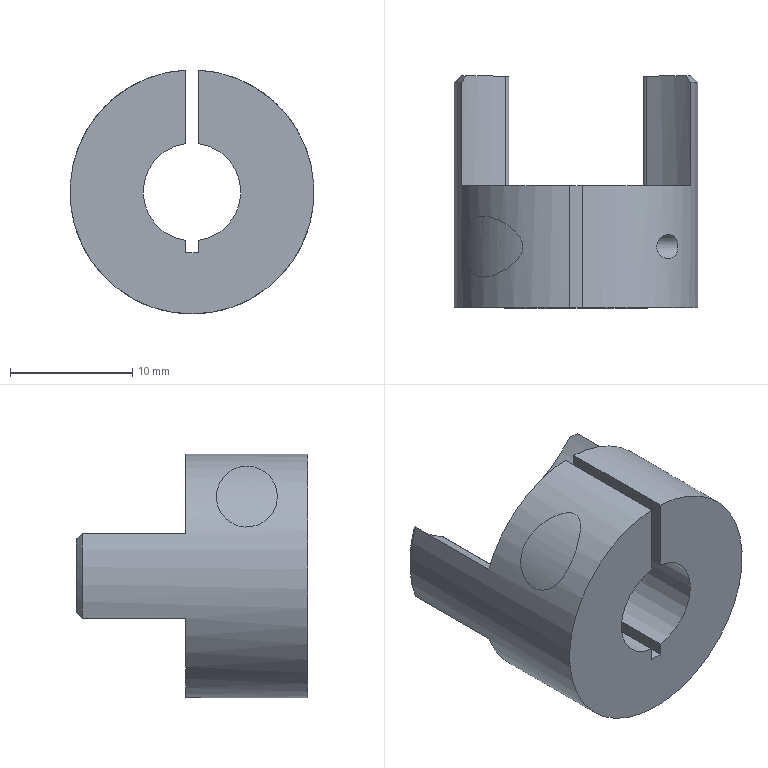Part | NX | features R-HUB_5003_022_GCJC20-BL-6-8 2 | 1 solid | 25 faces | box 20 x 19 x 19.987 mm | volume 2720 mm3 | cylinder 13 | plane 10 | cone 2 | commonest cylinder face diameters 24 x4 1 x2 8 x2 20 x2 2.013 x1 3 x1
STEP:
#1=CARTESIAN_POINT('',(-216.275,-588.6,-114.469));
#2=VERTEX_POINT('',#1);
#3=CARTESIAN_POINT('',(-216.275,-588.6,-106.531));
#4=VERTEX_POINT('',#3);
#5=CARTESIAN_POINT('',(-216.775,-588.6,-110.5));
#6=DIRECTION('',(0.,-1.,0.));
#7=DIRECTION('',(1.,0.,0.));
#8=AXIS2_PLACEMENT_3D('',#5,#6,#7);
#9=CIRCLE('',#8,4.);
#10=EDGE_CURVE('',#2,#4,#9,.T.);
#11=ORIENTED_EDGE('',*,*,#10,.T.);
#12=CARTESIAN_POINT('',(-216.275,-578.6,-106.531));
#13=VERTEX_POINT('',#12);
#14=CARTESIAN_POINT('',(-216.275,-569.599,-106.531));
#15=DIRECTION('',(0.,-1.,0.));
#16=VECTOR('',#15,1000.);
#17=LINE('',#14,#16);
#18=EDGE_CURVE('',#4,#13,#17,.F.);
#19=ORIENTED_EDGE('',*,*,#18,.T.);
#20=CARTESIAN_POINT('',(-216.275,-578.6,-114.469));
#21=VERTEX_POINT('',#20);
#22=CARTESIAN_POINT('',(-216.775,-578.6,-110.5));
#23=DIRECTION('',(0.,-1.,0.));
#24=DIRECTION('',(1.,0.,0.));
#25=AXIS2_PLACEMENT_3D('',#22,#23,#24);
#26=CIRCLE('',#25,4.);
#27=EDGE_CURVE('',#13,#21,#26,.F.);
#28=ORIENTED_EDGE('',*,*,#27,.T.);
#29=CARTESIAN_POINT('',(-216.275,-569.599,-114.469));
#30=DIRECTION('',(0.,-1.,0.));
#31=VECTOR('',#30,1000.);
#32=LINE('',#29,#31);
#33=EDGE_CURVE('',#21,#2,#32,.T.);
#34=ORIENTED_EDGE('',*,*,#33,.T.);
#35=EDGE_LOOP('',(#11,#19,#28,#34));
#36=FACE_BOUND('',#35,.T.);
#37=CARTESIAN_POINT('',(-216.775,-569.599,-110.5));
#38=DIRECTION('',(0.,-1.,0.));
#39=DIRECTION('',(1.,0.,0.));
#40=AXIS2_PLACEMENT_3D('',#37,#38,#39);
#41=CYLINDRICAL_SURFACE('',#40,4.);
#42=ADVANCED_FACE('',(#36),#41,.F.);
#43=CARTESIAN_POINT('',(-216.275,-588.6,-100.513));
#44=VERTEX_POINT('',#43);
#45=CARTESIAN_POINT('',(-217.275,-588.6,-100.513));
#46=VERTEX_POINT('',#45);
#47=CARTESIAN_POINT('',(-216.775,-588.6,-110.5));
#48=DIRECTION('',(0.,1.,0.));
#49=DIRECTION('',(-1.,0.,0.));
#50=AXIS2_PLACEMENT_3D('',#47,#48,#49);
#51=CIRCLE('',#50,10.);
#52=EDGE_CURVE('',#44,#46,#51,.T.);
#53=ORIENTED_EDGE('',*,*,#52,.F.);
#54=CARTESIAN_POINT('',(-216.275,-588.6,-110.5));
#55=DIRECTION('',(0.,0.,1.));
#56=VECTOR('',#55,1000.);
#57=LINE('',#54,#56);
#58=EDGE_CURVE('',#4,#44,#57,.T.);
#59=ORIENTED_EDGE('',*,*,#58,.F.);
#60=ORIENTED_EDGE('',*,*,#10,.F.);
#61=CARTESIAN_POINT('',(-216.275,-588.6,-115.5));
#62=VERTEX_POINT('',#61);
#63=CARTESIAN_POINT('',(-216.275,-588.6,-110.5));
#64=DIRECTION('',(0.,0.,1.));
#65=VECTOR('',#64,1000.);
#66=LINE('',#63,#65);
#67=EDGE_CURVE('',#62,#2,#66,.T.);
#68=ORIENTED_EDGE('',*,*,#67,.F.);
#69=CARTESIAN_POINT('',(-217.275,-588.6,-115.5));
#70=VERTEX_POINT('',#69);
#71=CARTESIAN_POINT('',(-216.775,-588.6,-115.5));
#72=DIRECTION('',(1.,0.,0.));
#73=VECTOR('',#72,1000.);
#74=LINE('',#71,#73);
#75=EDGE_CURVE('',#70,#62,#74,.T.);
#76=ORIENTED_EDGE('',*,*,#75,.F.);
#77=CARTESIAN_POINT('',(-217.275,-588.6,-114.469));
#78=VERTEX_POINT('',#77);
#79=CARTESIAN_POINT('',(-217.275,-588.6,-110.5));
#80=DIRECTION('',(0.,0.,-1.));
#81=VECTOR('',#80,1000.);
#82=LINE('',#79,#81);
#83=EDGE_CURVE('',#78,#70,#82,.T.);
#84=ORIENTED_EDGE('',*,*,#83,.F.);
#85=CARTESIAN_POINT('',(-217.275,-588.6,-106.531));
#86=VERTEX_POINT('',#85);
#87=CARTESIAN_POINT('',(-216.775,-588.6,-110.5));
#88=DIRECTION('',(0.,-1.,0.));
#89=DIRECTION('',(1.,0.,0.));
#90=AXIS2_PLACEMENT_3D('',#87,#88,#89);
#91=CIRCLE('',#90,4.);
#92=EDGE_CURVE('',#86,#78,#91,.T.);
#93=ORIENTED_EDGE('',*,*,#92,.F.);
#94=CARTESIAN_POINT('',(-217.275,-588.6,-110.5));
#95=DIRECTION('',(0.,0.,-1.));
#96=VECTOR('',#95,1000.);
#97=LINE('',#94,#96);
#98=EDGE_CURVE('',#46,#86,#97,.T.);
#99=ORIENTED_EDGE('',*,*,#98,.F.);
#100=EDGE_LOOP('',(#53,#59,#60,#68,#76,#84,#93,#99));
#101=FACE_BOUND('',#100,.T.);
#102=CARTESIAN_POINT('',(-216.775,-588.6,-110.5));
#103=DIRECTION('',(0.,1.,0.));
#104=DIRECTION('',(-1.,0.,0.));
#105=AXIS2_PLACEMENT_3D('',#102,#103,#104);
#106=PLANE('',#105);
#107=ADVANCED_FACE('',(#101),#106,.F.);
#108=CARTESIAN_POINT('',(-209.176,-584.606,-104.));
#109=VERTEX_POINT('',#108);
#110=CARTESIAN_POINT('',(-208.586,-584.456,-104.743));
#111=CARTESIAN_POINT('',(-209.17,-584.677,-103.982));
#112=CARTESIAN_POINT('',(-209.789,-584.474,-103.328));
#113=CARTESIAN_POINT('',(-210.332,-583.676,-102.85));
#114=CARTESIAN_POINT('',(-209.879,-582.783,-103.244));
#115=CARTESIAN_POINT('',(-209.245,-582.531,-103.895));
#116=CARTESIAN_POINT('',(-208.657,-582.678,-104.64));
#117=CARTESIAN_POINT('',(-208.32,-583.521,-105.161));
#118=CARTESIAN_POINT('',(-208.586,-584.456,-104.743));
#119=CARTESIAN_POINT('',(-209.17,-584.677,-103.982));
#120=CARTESIAN_POINT('',(-209.789,-584.474,-103.328));
#121=B_SPLINE_CURVE_WITH_KNOTS('',3,(#110,#111,#112,#113,#114,#115,#116,#117,#118,#119,#120),.UNSPECIFIED.,.T.,.F.,(1,1,1,1,1,1,1,1,1,1,1,1,1,1,1),(-0.002757,-0.001838,-0.0009191,0.,0.0009191,0.001838,0.002757,0.003677,0.004596,0.005515,0.006434,0.007353,0.008272,0.009191,0.01011),.UNSPECIFIED.);
#122=EDGE_CURVE('',#109,#109,#121,.T.);
#123=ORIENTED_EDGE('',*,*,#122,.T.);
#124=EDGE_LOOP('',(#123));
#125=FACE_BOUND('',#124,.T.);
#126=CARTESIAN_POINT('',(-224.374,-586.1,-104.));
#127=VERTEX_POINT('',#126);
#128=CARTESIAN_POINT('',(-223.569,-585.992,-103.133));
#129=CARTESIAN_POINT('',(-224.667,-586.211,-104.258));
#130=CARTESIAN_POINT('',(-225.77,-585.644,-106.008));
#131=CARTESIAN_POINT('',(-226.096,-583.084,-106.883));
#132=CARTESIAN_POINT('',(-225.39,-581.073,-105.242));
#133=CARTESIAN_POINT('',(-224.083,-581.028,-103.593));
#134=CARTESIAN_POINT('',(-222.942,-581.475,-102.603));
#135=CARTESIAN_POINT('',(-222.075,-582.027,-101.999));
#136=CARTESIAN_POINT('',(-221.398,-582.684,-101.628));
#137=CARTESIAN_POINT('',(-221.094,-583.426,-101.481));
#138=CARTESIAN_POINT('',(-221.2,-584.249,-101.531));
#139=CARTESIAN_POINT('',(-221.847,-584.986,-101.863));
#140=CARTESIAN_POINT('',(-222.698,-585.592,-102.419));
#141=CARTESIAN_POINT('',(-223.569,-585.992,-103.133));
#142=CARTESIAN_POINT('',(-224.667,-586.211,-104.258));
#143=CARTESIAN_POINT('',(-225.77,-585.644,-106.008));
#144=B_SPLINE_CURVE_WITH_KNOTS('',3,(#128,#129,#130,#131,#132,#133,#134,#135,#136,#137,#138,#139,#140,#141,#142,#143),.UNSPECIFIED.,.T.,.F.,(1,1,1,1,1,1,1,1,1,1,1,1,1,1,1,1,1,1,1,1),(-0.003531,-0.002354,-0.001177,0.,0.002354,0.004707,0.007061,0.009415,0.01059,0.01177,0.01295,0.01353,0.01412,0.0153,0.01648,0.01765,0.01883,0.02118,0.02354,0.02589),.UNSPECIFIED.);
#145=EDGE_CURVE('',#127,#127,#144,.T.);
#146=ORIENTED_EDGE('',*,*,#145,.T.);
#147=EDGE_LOOP('',(#146));
#148=FACE_BOUND('',#147,.T.);
#149=CARTESIAN_POINT('',(-216.275,-578.6,-100.513));
#150=VERTEX_POINT('',#149);
#151=CARTESIAN_POINT('',(-207.399,-578.6,-107.023));
#152=VERTEX_POINT('',#151);
#153=CARTESIAN_POINT('',(-216.775,-578.6,-110.5));
#154=DIRECTION('',(0.,1.,0.));
#155=DIRECTION('',(-1.,0.,0.));
#156=AXIS2_PLACEMENT_3D('',#153,#154,#155);
#157=CIRCLE('',#156,10.);
#158=EDGE_CURVE('',#150,#152,#157,.T.);
#159=ORIENTED_EDGE('',*,*,#158,.F.);
#160=CARTESIAN_POINT('',(-216.275,-578.6,-100.513));
#161=DIRECTION('',(0.,-1.,0.));
#162=VECTOR('',#161,1000.);
#163=LINE('',#160,#162);
#164=EDGE_CURVE('',#150,#44,#163,.T.);
#165=ORIENTED_EDGE('',*,*,#164,.T.);
#166=ORIENTED_EDGE('',*,*,#52,.T.);
#167=CARTESIAN_POINT('',(-217.275,-578.6,-100.513));
#168=VERTEX_POINT('',#167);
#169=CARTESIAN_POINT('',(-217.275,-578.6,-100.513));
#170=DIRECTION('',(0.,-1.,0.));
#171=VECTOR('',#170,1000.);
#172=LINE('',#169,#171);
#173=EDGE_CURVE('',#168,#46,#172,.T.);
#174=ORIENTED_EDGE('',*,*,#173,.F.);
#175=CARTESIAN_POINT('',(-226.151,-578.6,-107.023));
#176=VERTEX_POINT('',#175);
#177=CARTESIAN_POINT('',(-216.775,-578.6,-110.5));
#178=DIRECTION('',(0.,1.,0.));
#179=DIRECTION('',(-1.,0.,0.));
#180=AXIS2_PLACEMENT_3D('',#177,#178,#179);
#181=CIRCLE('',#180,10.);
#182=EDGE_CURVE('',#176,#168,#181,.T.);
#183=ORIENTED_EDGE('',*,*,#182,.F.);
#184=CARTESIAN_POINT('',(-226.151,-570.1,-107.023));
#185=VERTEX_POINT('',#184);
#186=CARTESIAN_POINT('',(-226.151,-569.6,-107.023));
#187=DIRECTION('',(0.,-1.,0.));
#188=VECTOR('',#187,1000.);
#189=LINE('',#186,#188);
#190=EDGE_CURVE('',#185,#176,#189,.T.);
#191=ORIENTED_EDGE('',*,*,#190,.F.);
#192=CARTESIAN_POINT('',(-226.151,-570.1,-113.977));
#193=VERTEX_POINT('',#192);
#194=CARTESIAN_POINT('',(-216.775,-570.1,-110.5));
#195=DIRECTION('',(0.,-1.,0.));
#196=DIRECTION('',(1.,0.,0.));
#197=AXIS2_PLACEMENT_3D('',#194,#195,#196);
#198=CIRCLE('',#197,10.);
#199=EDGE_CURVE('',#185,#193,#198,.T.);
#200=ORIENTED_EDGE('',*,*,#199,.T.);
#201=CARTESIAN_POINT('',(-226.151,-578.6,-113.977));
#202=VERTEX_POINT('',#201);
#203=CARTESIAN_POINT('',(-226.151,-569.6,-113.977));
#204=DIRECTION('',(0.,-1.,0.));
#205=VECTOR('',#204,1000.);
#206=LINE('',#203,#205);
#207=EDGE_CURVE('',#193,#202,#206,.T.);
#208=ORIENTED_EDGE('',*,*,#207,.T.);
#209=CARTESIAN_POINT('',(-207.399,-578.6,-113.977));
#210=VERTEX_POINT('',#209);
#211=CARTESIAN_POINT('',(-216.775,-578.6,-110.5));
#212=DIRECTION('',(0.,1.,0.));
#213=DIRECTION('',(-1.,0.,0.));
#214=AXIS2_PLACEMENT_3D('',#211,#212,#213);
#215=CIRCLE('',#214,10.);
#216=EDGE_CURVE('',#210,#202,#215,.T.);
#217=ORIENTED_EDGE('',*,*,#216,.F.);
#218=CARTESIAN_POINT('',(-207.399,-570.1,-113.977));
#219=VERTEX_POINT('',#218);
#220=CARTESIAN_POINT('',(-207.399,-569.6,-113.977));
#221=DIRECTION('',(0.,-1.,0.));
#222=VECTOR('',#221,1000.);
#223=LINE('',#220,#222);
#224=EDGE_CURVE('',#219,#210,#223,.T.);
#225=ORIENTED_EDGE('',*,*,#224,.F.);
#226=CARTESIAN_POINT('',(-207.399,-570.1,-107.023));
#227=VERTEX_POINT('',#226);
#228=CARTESIAN_POINT('',(-216.775,-570.1,-110.5));
#229=DIRECTION('',(0.,-1.,0.));
#230=DIRECTION('',(1.,0.,0.));
#231=AXIS2_PLACEMENT_3D('',#228,#229,#230);
#232=CIRCLE('',#231,10.);
#233=EDGE_CURVE('',#219,#227,#232,.T.);
#234=ORIENTED_EDGE('',*,*,#233,.T.);
#235=CARTESIAN_POINT('',(-207.399,-569.6,-107.023));
#236=DIRECTION('',(0.,-1.,0.));
#237=VECTOR('',#236,1000.);
#238=LINE('',#235,#237);
#239=EDGE_CURVE('',#227,#152,#238,.T.);
#240=ORIENTED_EDGE('',*,*,#239,.T.);
#241=EDGE_LOOP('',(#159,#165,#166,#174,#183,#191,#200,#208,#217,#225,#234,#240));
#242=FACE_BOUND('',#241,.T.);
#243=CARTESIAN_POINT('',(-216.775,-568.65,-110.5));
#244=DIRECTION('',(0.,1.,0.));
#245=DIRECTION('',(-1.,0.,0.));
#246=AXIS2_PLACEMENT_3D('',#243,#244,#245);
#247=CYLINDRICAL_SURFACE('',#246,10.);
#248=ADVANCED_FACE('',(#125,#148,#242),#247,.T.);
#249=ORIENTED_EDGE('',*,*,#27,.F.);
#250=CARTESIAN_POINT('',(-216.275,-578.6,-110.5));
#251=DIRECTION('',(0.,0.,1.));
#252=VECTOR('',#251,1000.);
#253=LINE('',#250,#252);
#254=EDGE_CURVE('',#13,#150,#253,.T.);
#255=ORIENTED_EDGE('',*,*,#254,.T.);
#256=ORIENTED_EDGE('',*,*,#158,.T.);
#257=CARTESIAN_POINT('',(-211.015,-578.6,-110.061));
#258=VERTEX_POINT('',#257);
#259=CARTESIAN_POINT('',(-216.775,-578.6,-99.534));
#260=DIRECTION('',(0.,1.,0.));
#261=DIRECTION('',(1.,0.,0.));
#262=AXIS2_PLACEMENT_3D('',#259,#260,#261);
#263=CIRCLE('',#262,12.);
#264=EDGE_CURVE('',#152,#258,#263,.T.);
#265=ORIENTED_EDGE('',*,*,#264,.T.);
#266=CARTESIAN_POINT('',(-211.015,-578.6,-110.939));
#267=VERTEX_POINT('',#266);
#268=CARTESIAN_POINT('',(-210.775,-578.6,-110.5));
#269=DIRECTION('',(0.,-1.,0.));
#270=DIRECTION('',(1.,0.,0.));
#271=AXIS2_PLACEMENT_3D('',#268,#269,#270);
#272=CIRCLE('',#271,0.5);
#273=EDGE_CURVE('',#258,#267,#272,.T.);
#274=ORIENTED_EDGE('',*,*,#273,.T.);
#275=CARTESIAN_POINT('',(-216.775,-578.6,-121.466));
#276=DIRECTION('',(0.,1.,0.));
#277=DIRECTION('',(1.,0.,0.));
#278=AXIS2_PLACEMENT_3D('',#275,#276,#277);
#279=CIRCLE('',#278,12.);
#280=EDGE_CURVE('',#267,#210,#279,.T.);
#281=ORIENTED_EDGE('',*,*,#280,.T.);
#282=ORIENTED_EDGE('',*,*,#216,.T.);
#283=CARTESIAN_POINT('',(-222.535,-578.6,-110.939));
#284=VERTEX_POINT('',#283);
#285=CARTESIAN_POINT('',(-216.775,-578.6,-121.466));
#286=DIRECTION('',(0.,1.,0.));
#287=DIRECTION('',(1.,0.,0.));
#288=AXIS2_PLACEMENT_3D('',#285,#286,#287);
#289=CIRCLE('',#288,12.);
#290=EDGE_CURVE('',#202,#284,#289,.T.);
#291=ORIENTED_EDGE('',*,*,#290,.T.);
#292=CARTESIAN_POINT('',(-222.535,-578.6,-110.061));
#293=VERTEX_POINT('',#292);
#294=CARTESIAN_POINT('',(-222.775,-578.6,-110.5));
#295=DIRECTION('',(0.,-1.,0.));
#296=DIRECTION('',(1.,0.,0.));
#297=AXIS2_PLACEMENT_3D('',#294,#295,#296);
#298=CIRCLE('',#297,0.5);
#299=EDGE_CURVE('',#284,#293,#298,.T.);
#300=ORIENTED_EDGE('',*,*,#299,.T.);
#301=CARTESIAN_POINT('',(-216.775,-578.6,-99.534));
#302=DIRECTION('',(0.,1.,0.));
#303=DIRECTION('',(1.,0.,0.));
#304=AXIS2_PLACEMENT_3D('',#301,#302,#303);
#305=CIRCLE('',#304,12.);
#306=EDGE_CURVE('',#293,#176,#305,.T.);
#307=ORIENTED_EDGE('',*,*,#306,.T.);
#308=ORIENTED_EDGE('',*,*,#182,.T.);
#309=CARTESIAN_POINT('',(-217.275,-578.6,-106.531));
#310=VERTEX_POINT('',#309);
#311=CARTESIAN_POINT('',(-217.275,-578.6,-110.5));
#312=DIRECTION('',(0.,0.,-1.));
#313=VECTOR('',#312,1000.);
#314=LINE('',#311,#313);
#315=EDGE_CURVE('',#168,#310,#314,.T.);
#316=ORIENTED_EDGE('',*,*,#315,.T.);
#317=CARTESIAN_POINT('',(-217.275,-578.6,-114.469));
#318=VERTEX_POINT('',#317);
#319=CARTESIAN_POINT('',(-216.775,-578.6,-110.5));
#320=DIRECTION('',(0.,-1.,0.));
#321=DIRECTION('',(1.,0.,0.));
#322=AXIS2_PLACEMENT_3D('',#319,#320,#321);
#323=CIRCLE('',#322,4.);
#324=EDGE_CURVE('',#318,#310,#323,.F.);
#325=ORIENTED_EDGE('',*,*,#324,.F.);
#326=CARTESIAN_POINT('',(-217.275,-578.6,-115.5));
#327=VERTEX_POINT('',#326);
#328=CARTESIAN_POINT('',(-217.275,-578.6,-110.5));
#329=DIRECTION('',(0.,0.,-1.));
#330=VECTOR('',#329,1000.);
#331=LINE('',#328,#330);
#332=EDGE_CURVE('',#318,#327,#331,.T.);
#333=ORIENTED_EDGE('',*,*,#332,.T.);
#334=CARTESIAN_POINT('',(-216.275,-578.6,-115.5));
#335=VERTEX_POINT('',#334);
#336=CARTESIAN_POINT('',(-216.775,-578.6,-115.5));
#337=DIRECTION('',(1.,0.,0.));
#338=VECTOR('',#337,1000.);
#339=LINE('',#336,#338);
#340=EDGE_CURVE('',#327,#335,#339,.T.);
#341=ORIENTED_EDGE('',*,*,#340,.T.);
#342=CARTESIAN_POINT('',(-216.275,-578.6,-110.5));
#343=DIRECTION('',(0.,0.,1.));
#344=VECTOR('',#343,1000.);
#345=LINE('',#342,#344);
#346=EDGE_CURVE('',#335,#21,#345,.T.);
#347=ORIENTED_EDGE('',*,*,#346,.T.);
#348=EDGE_LOOP('',(#249,#255,#256,#265,#274,#281,#282,#291,#300,#307,#308,#316,#325,#333,#341,#347));
#349=FACE_BOUND('',#348,.T.);
#350=CARTESIAN_POINT('',(-216.775,-578.6,-110.5));
#351=DIRECTION('',(0.,-1.,0.));
#352=DIRECTION('',(1.,0.,0.));
#353=AXIS2_PLACEMENT_3D('',#350,#351,#352);
#354=PLANE('',#353);
#355=ADVANCED_FACE('',(#349),#354,.F.);
#356=ORIENTED_EDGE('',*,*,#299,.F.);
#357=CARTESIAN_POINT('',(-222.535,-569.6,-110.939));
#358=VERTEX_POINT('',#357);
#359=CARTESIAN_POINT('',(-222.535,-569.6,-110.939));
#360=DIRECTION('',(0.,-1.,0.));
#361=VECTOR('',#360,1000.);
#362=LINE('',#359,#361);
#363=EDGE_CURVE('',#358,#284,#362,.T.);
#364=ORIENTED_EDGE('',*,*,#363,.F.);
#365=CARTESIAN_POINT('',(-222.535,-569.6,-110.061));
#366=VERTEX_POINT('',#365);
#367=CARTESIAN_POINT('',(-222.775,-569.6,-110.5));
#368=DIRECTION('',(0.,-1.,0.));
#369=DIRECTION('',(1.,0.,0.));
#370=AXIS2_PLACEMENT_3D('',#367,#368,#369);
#371=CIRCLE('',#370,0.5);
#372=EDGE_CURVE('',#358,#366,#371,.T.);
#373=ORIENTED_EDGE('',*,*,#372,.T.);
#374=CARTESIAN_POINT('',(-222.535,-569.6,-110.061));
#375=DIRECTION('',(0.,-1.,0.));
#376=VECTOR('',#375,1000.);
#377=LINE('',#374,#376);
#378=EDGE_CURVE('',#366,#293,#377,.T.);
#379=ORIENTED_EDGE('',*,*,#378,.T.);
#380=EDGE_LOOP('',(#356,#364,#373,#379));
#381=FACE_BOUND('',#380,.T.);
#382=CARTESIAN_POINT('',(-222.775,-569.6,-110.5));
#383=DIRECTION('',(0.,-1.,0.));
#384=DIRECTION('',(1.,0.,0.));
#385=AXIS2_PLACEMENT_3D('',#382,#383,#384);
#386=CYLINDRICAL_SURFACE('',#385,0.5);
#387=ADVANCED_FACE('',(#381),#386,.T.);
#388=ORIENTED_EDGE('',*,*,#207,.F.);
#389=CARTESIAN_POINT('',(-225.778,-569.6,-113.532));
#390=VERTEX_POINT('',#389);
#391=CARTESIAN_POINT('',(-226.151,-570.1,-113.977));
#392=CARTESIAN_POINT('',(-226.03,-569.934,-113.825));
#393=CARTESIAN_POINT('',(-225.906,-569.767,-113.677));
#394=CARTESIAN_POINT('',(-225.778,-569.6,-113.532));
#395=B_SPLINE_CURVE_WITH_KNOTS('',3,(#391,#392,#393,#394),.UNSPECIFIED.,.F.,.F.,(4,4),(0.,0.000766),.UNSPECIFIED.);
#396=EDGE_CURVE('',#193,#390,#395,.T.);
#397=ORIENTED_EDGE('',*,*,#396,.T.);
#398=CARTESIAN_POINT('',(-216.775,-569.6,-121.466));
#399=DIRECTION('',(0.,1.,0.));
#400=DIRECTION('',(1.,0.,0.));
#401=AXIS2_PLACEMENT_3D('',#398,#399,#400);
#402=CIRCLE('',#401,12.);
#403=EDGE_CURVE('',#390,#358,#402,.T.);
#404=ORIENTED_EDGE('',*,*,#403,.T.);
#405=ORIENTED_EDGE('',*,*,#363,.T.);
#406=ORIENTED_EDGE('',*,*,#290,.F.);
#407=EDGE_LOOP('',(#388,#397,#404,#405,#406));
#408=FACE_BOUND('',#407,.T.);
#409=CARTESIAN_POINT('',(-216.775,-569.6,-121.466));
#410=DIRECTION('',(0.,-1.,0.));
#411=DIRECTION('',(1.,0.,0.));
#412=AXIS2_PLACEMENT_3D('',#409,#410,#411);
#413=CYLINDRICAL_SURFACE('',#412,12.);
#414=ADVANCED_FACE('',(#408),#413,.F.);
#415=CARTESIAN_POINT('',(-225.778,-569.6,-107.468));
#416=VERTEX_POINT('',#415);
#417=CARTESIAN_POINT('',(-216.775,-569.6,-99.534));
#418=DIRECTION('',(0.,1.,0.));
#419=DIRECTION('',(1.,0.,0.));
#420=AXIS2_PLACEMENT_3D('',#417,#418,#419);
#421=CIRCLE('',#420,12.);
#422=EDGE_CURVE('',#366,#416,#421,.T.);
#423=ORIENTED_EDGE('',*,*,#422,.T.);
#424=CARTESIAN_POINT('',(-225.778,-569.6,-107.468));
#425=CARTESIAN_POINT('',(-225.906,-569.767,-107.323));
#426=CARTESIAN_POINT('',(-226.03,-569.934,-107.175));
#427=CARTESIAN_POINT('',(-226.151,-570.1,-107.023));
#428=B_SPLINE_CURVE_WITH_KNOTS('',3,(#424,#425,#426,#427),.UNSPECIFIED.,.F.,.F.,(4,4),(0.,0.000766),.UNSPECIFIED.);
#429=EDGE_CURVE('',#416,#185,#428,.T.);
#430=ORIENTED_EDGE('',*,*,#429,.T.);
#431=ORIENTED_EDGE('',*,*,#190,.T.);
#432=ORIENTED_EDGE('',*,*,#306,.F.);
#433=ORIENTED_EDGE('',*,*,#378,.F.);
#434=EDGE_LOOP('',(#423,#430,#431,#432,#433));
#435=FACE_BOUND('',#434,.T.);
#436=CARTESIAN_POINT('',(-216.775,-569.6,-99.534));
#437=DIRECTION('',(0.,-1.,0.));
#438=DIRECTION('',(1.,0.,0.));
#439=AXIS2_PLACEMENT_3D('',#436,#437,#438);
#440=CYLINDRICAL_SURFACE('',#439,12.);
#441=ADVANCED_FACE('',(#435),#440,.F.);
#442=ORIENTED_EDGE('',*,*,#403,.F.);
#443=CARTESIAN_POINT('',(-216.775,-569.6,-110.5));
#444=DIRECTION('',(0.,-1.,0.));
#445=DIRECTION('',(1.,0.,0.));
#446=AXIS2_PLACEMENT_3D('',#443,#444,#445);
#447=CIRCLE('',#446,9.5);
#448=EDGE_CURVE('',#390,#416,#447,.F.);
#449=ORIENTED_EDGE('',*,*,#448,.T.);
#450=ORIENTED_EDGE('',*,*,#422,.F.);
#451=ORIENTED_EDGE('',*,*,#372,.F.);
#452=EDGE_LOOP('',(#442,#449,#450,#451));
#453=FACE_BOUND('',#452,.T.);
#454=CARTESIAN_POINT('',(-219.775,-569.6,-105.017));
#455=DIRECTION('',(0.,-1.,0.));
#456=DIRECTION('',(1.,0.,0.));
#457=AXIS2_PLACEMENT_3D('',#454,#455,#456);
#458=PLANE('',#457);
#459=ADVANCED_FACE('',(#453),#458,.F.);
#460=ORIENTED_EDGE('',*,*,#273,.F.);
#461=CARTESIAN_POINT('',(-211.015,-569.6,-110.061));
#462=VERTEX_POINT('',#461);
#463=CARTESIAN_POINT('',(-211.015,-569.6,-110.061));
#464=DIRECTION('',(0.,-1.,0.));
#465=VECTOR('',#464,1000.);
#466=LINE('',#463,#465);
#467=EDGE_CURVE('',#462,#258,#466,.T.);
#468=ORIENTED_EDGE('',*,*,#467,.F.);
#469=CARTESIAN_POINT('',(-211.015,-569.6,-110.939));
#470=VERTEX_POINT('',#469);
#471=CARTESIAN_POINT('',(-210.775,-569.6,-110.5));
#472=DIRECTION('',(0.,-1.,0.));
#473=DIRECTION('',(1.,0.,0.));
#474=AXIS2_PLACEMENT_3D('',#471,#472,#473);
#475=CIRCLE('',#474,0.5);
#476=EDGE_CURVE('',#462,#470,#475,.T.);
#477=ORIENTED_EDGE('',*,*,#476,.T.);
#478=CARTESIAN_POINT('',(-211.015,-569.6,-110.939));
#479=DIRECTION('',(0.,-1.,0.));
#480=VECTOR('',#479,1000.);
#481=LINE('',#478,#480);
#482=EDGE_CURVE('',#470,#267,#481,.T.);
#483=ORIENTED_EDGE('',*,*,#482,.T.);
#484=EDGE_LOOP('',(#460,#468,#477,#483));
#485=FACE_BOUND('',#484,.T.);
#486=CARTESIAN_POINT('',(-210.775,-569.6,-110.5));
#487=DIRECTION('',(0.,-1.,0.));
#488=DIRECTION('',(1.,0.,0.));
#489=AXIS2_PLACEMENT_3D('',#486,#487,#488);
#490=CYLINDRICAL_SURFACE('',#489,0.5);
#491=ADVANCED_FACE('',(#485),#490,.T.);
#492=ORIENTED_EDGE('',*,*,#239,.F.);
#493=CARTESIAN_POINT('',(-207.772,-569.6,-107.468));
#494=VERTEX_POINT('',#493);
#495=CARTESIAN_POINT('',(-207.399,-570.1,-107.023));
#496=CARTESIAN_POINT('',(-207.52,-569.934,-107.175));
#497=CARTESIAN_POINT('',(-207.644,-569.767,-107.323));
#498=CARTESIAN_POINT('',(-207.772,-569.6,-107.468));
#499=B_SPLINE_CURVE_WITH_KNOTS('',3,(#495,#496,#497,#498),.UNSPECIFIED.,.F.,.F.,(4,4),(0.,0.000766),.UNSPECIFIED.);
#500=EDGE_CURVE('',#227,#494,#499,.T.);
#501=ORIENTED_EDGE('',*,*,#500,.T.);
#502=CARTESIAN_POINT('',(-216.775,-569.6,-99.534));
#503=DIRECTION('',(0.,1.,0.));
#504=DIRECTION('',(1.,0.,0.));
#505=AXIS2_PLACEMENT_3D('',#502,#503,#504);
#506=CIRCLE('',#505,12.);
#507=EDGE_CURVE('',#494,#462,#506,.T.);
#508=ORIENTED_EDGE('',*,*,#507,.T.);
#509=ORIENTED_EDGE('',*,*,#467,.T.);
#510=ORIENTED_EDGE('',*,*,#264,.F.);
#511=EDGE_LOOP('',(#492,#501,#508,#509,#510));
#512=FACE_BOUND('',#511,.T.);
#513=CARTESIAN_POINT('',(-216.775,-569.6,-99.534));
#514=DIRECTION('',(0.,-1.,0.));
#515=DIRECTION('',(1.,0.,0.));
#516=AXIS2_PLACEMENT_3D('',#513,#514,#515);
#517=CYLINDRICAL_SURFACE('',#516,12.);
#518=ADVANCED_FACE('',(#512),#517,.F.);
#519=CARTESIAN_POINT('',(-207.772,-569.6,-113.532));
#520=VERTEX_POINT('',#519);
#521=CARTESIAN_POINT('',(-216.775,-569.6,-121.466));
#522=DIRECTION('',(0.,1.,0.));
#523=DIRECTION('',(1.,0.,0.));
#524=AXIS2_PLACEMENT_3D('',#521,#522,#523);
#525=CIRCLE('',#524,12.);
#526=EDGE_CURVE('',#470,#520,#525,.T.);
#527=ORIENTED_EDGE('',*,*,#526,.T.);
#528=CARTESIAN_POINT('',(-207.772,-569.6,-113.532));
#529=CARTESIAN_POINT('',(-207.644,-569.767,-113.677));
#530=CARTESIAN_POINT('',(-207.52,-569.934,-113.825));
#531=CARTESIAN_POINT('',(-207.399,-570.1,-113.977));
#532=B_SPLINE_CURVE_WITH_KNOTS('',3,(#528,#529,#530,#531),.UNSPECIFIED.,.F.,.F.,(4,4),(0.,0.000766),.UNSPECIFIED.);
#533=EDGE_CURVE('',#520,#219,#532,.T.);
#534=ORIENTED_EDGE('',*,*,#533,.T.);
#535=ORIENTED_EDGE('',*,*,#224,.T.);
#536=ORIENTED_EDGE('',*,*,#280,.F.);
#537=ORIENTED_EDGE('',*,*,#482,.F.);
#538=EDGE_LOOP('',(#527,#534,#535,#536,#537));
#539=FACE_BOUND('',#538,.T.);
#540=CARTESIAN_POINT('',(-216.775,-569.6,-121.466));
#541=DIRECTION('',(0.,-1.,0.));
#542=DIRECTION('',(1.,0.,0.));
#543=AXIS2_PLACEMENT_3D('',#540,#541,#542);
#544=CYLINDRICAL_SURFACE('',#543,12.);
#545=ADVANCED_FACE('',(#539),#544,.F.);
#546=ORIENTED_EDGE('',*,*,#507,.F.);
#547=CARTESIAN_POINT('',(-216.775,-569.6,-110.5));
#548=DIRECTION('',(0.,-1.,0.));
#549=DIRECTION('',(1.,0.,0.));
#550=AXIS2_PLACEMENT_3D('',#547,#548,#549);
#551=CIRCLE('',#550,9.5);
#552=EDGE_CURVE('',#494,#520,#551,.F.);
#553=ORIENTED_EDGE('',*,*,#552,.T.);
#554=ORIENTED_EDGE('',*,*,#526,.F.);
#555=ORIENTED_EDGE('',*,*,#476,.F.);
#556=EDGE_LOOP('',(#546,#553,#554,#555));
#557=FACE_BOUND('',#556,.T.);
#558=CARTESIAN_POINT('',(-213.775,-569.6,-115.983));
#559=DIRECTION('',(0.,-1.,0.));
#560=DIRECTION('',(1.,0.,0.));
#561=AXIS2_PLACEMENT_3D('',#558,#559,#560);
#562=PLANE('',#561);
#563=ADVANCED_FACE('',(#557),#562,.F.);
#564=ORIENTED_EDGE('',*,*,#533,.F.);
#565=ORIENTED_EDGE('',*,*,#552,.F.);
#566=ORIENTED_EDGE('',*,*,#500,.F.);
#567=ORIENTED_EDGE('',*,*,#233,.F.);
#568=EDGE_LOOP('',(#564,#565,#566,#567));
#569=FACE_BOUND('',#568,.T.);
#570=CARTESIAN_POINT('',(-216.775,-570.1,-110.5));
#571=DIRECTION('',(0.,-1.,0.));
#572=DIRECTION('',(1.,0.,0.));
#573=AXIS2_PLACEMENT_3D('',#570,#571,#572);
#574=CONICAL_SURFACE('',#573,10.,0.7854);
#575=ADVANCED_FACE('',(#569),#574,.T.);
#576=ORIENTED_EDGE('',*,*,#429,.F.);
#577=ORIENTED_EDGE('',*,*,#448,.F.);
#578=ORIENTED_EDGE('',*,*,#396,.F.);
#579=ORIENTED_EDGE('',*,*,#199,.F.);
#580=EDGE_LOOP('',(#576,#577,#578,#579));
#581=FACE_BOUND('',#580,.T.);
#582=CARTESIAN_POINT('',(-216.775,-570.1,-110.5));
#583=DIRECTION('',(0.,-1.,0.));
#584=DIRECTION('',(1.,0.,0.));
#585=AXIS2_PLACEMENT_3D('',#582,#583,#584);
#586=CONICAL_SURFACE('',#585,10.,0.7854);
#587=ADVANCED_FACE('',(#581),#586,.T.);
#588=ORIENTED_EDGE('',*,*,#92,.T.);
#589=CARTESIAN_POINT('',(-217.275,-569.599,-114.469));
#590=DIRECTION('',(0.,-1.,0.));
#591=VECTOR('',#590,1000.);
#592=LINE('',#589,#591);
#593=EDGE_CURVE('',#78,#318,#592,.F.);
#594=ORIENTED_EDGE('',*,*,#593,.T.);
#595=ORIENTED_EDGE('',*,*,#324,.T.);
#596=CARTESIAN_POINT('',(-217.275,-569.599,-106.531));
#597=DIRECTION('',(0.,-1.,0.));
#598=VECTOR('',#597,1000.);
#599=LINE('',#596,#598);
#600=EDGE_CURVE('',#310,#86,#599,.T.);
#601=ORIENTED_EDGE('',*,*,#600,.T.);
#602=EDGE_LOOP('',(#588,#594,#595,#601));
#603=FACE_BOUND('',#602,.T.);
#604=CARTESIAN_POINT('',(-216.775,-569.599,-110.5));
#605=DIRECTION('',(0.,-1.,0.));
#606=DIRECTION('',(1.,0.,0.));
#607=AXIS2_PLACEMENT_3D('',#604,#605,#606);
#608=CYLINDRICAL_SURFACE('',#607,4.);
#609=ADVANCED_FACE('',(#603),#608,.F.);
#610=CARTESIAN_POINT('',(-217.275,-583.6,-105.5));
#611=VERTEX_POINT('',#610);
#612=CARTESIAN_POINT('',(-217.275,-583.6,-104.));
#613=DIRECTION('',(-1.,0.,0.));
#614=DIRECTION('',(0.,0.,-1.));
#615=AXIS2_PLACEMENT_3D('',#612,#613,#614);
#616=CIRCLE('',#615,1.5);
#617=EDGE_CURVE('',#611,#611,#616,.T.);
#618=ORIENTED_EDGE('',*,*,#617,.T.);
#619=EDGE_LOOP('',(#618));
#620=FACE_BOUND('',#619,.T.);
#621=ORIENTED_EDGE('',*,*,#315,.F.);
#622=ORIENTED_EDGE('',*,*,#173,.T.);
#623=ORIENTED_EDGE('',*,*,#98,.T.);
#624=ORIENTED_EDGE('',*,*,#600,.F.);
#625=EDGE_LOOP('',(#621,#622,#623,#624));
#626=FACE_BOUND('',#625,.T.);
#627=CARTESIAN_POINT('',(-217.275,-578.6,-110.5));
#628=DIRECTION('',(-1.,0.,0.));
#629=DIRECTION('',(0.,0.,-1.));
#630=AXIS2_PLACEMENT_3D('',#627,#628,#629);
#631=PLANE('',#630);
#632=ADVANCED_FACE('',(#620,#626),#631,.F.);
#633=ORIENTED_EDGE('',*,*,#346,.F.);
#634=CARTESIAN_POINT('',(-216.275,-578.6,-115.5));
#635=DIRECTION('',(0.,-1.,0.));
#636=VECTOR('',#635,1000.);
#637=LINE('',#634,#636);
#638=EDGE_CURVE('',#335,#62,#637,.T.);
#639=ORIENTED_EDGE('',*,*,#638,.T.);
#640=ORIENTED_EDGE('',*,*,#67,.T.);
#641=ORIENTED_EDGE('',*,*,#33,.F.);
#642=EDGE_LOOP('',(#633,#639,#640,#641));
#643=FACE_BOUND('',#642,.T.);
#644=CARTESIAN_POINT('',(-216.275,-578.6,-110.5));
#645=DIRECTION('',(1.,0.,0.));
#646=DIRECTION('',(0.,0.,1.));
#647=AXIS2_PLACEMENT_3D('',#644,#645,#646);
#648=PLANE('',#647);
#649=ADVANCED_FACE('',(#643),#648,.F.);
#650=ORIENTED_EDGE('',*,*,#83,.T.);
#651=CARTESIAN_POINT('',(-217.275,-578.6,-115.5));
#652=DIRECTION('',(0.,-1.,0.));
#653=VECTOR('',#652,1000.);
#654=LINE('',#651,#653);
#655=EDGE_CURVE('',#327,#70,#654,.T.);
#656=ORIENTED_EDGE('',*,*,#655,.F.);
#657=ORIENTED_EDGE('',*,*,#332,.F.);
#658=ORIENTED_EDGE('',*,*,#593,.F.);
#659=EDGE_LOOP('',(#650,#656,#657,#658));
#660=FACE_BOUND('',#659,.T.);
#661=CARTESIAN_POINT('',(-217.275,-578.6,-110.5));
#662=DIRECTION('',(-1.,0.,0.));
#663=DIRECTION('',(0.,0.,-1.));
#664=AXIS2_PLACEMENT_3D('',#661,#662,#663);
#665=PLANE('',#664);
#666=ADVANCED_FACE('',(#660),#665,.F.);
#667=ORIENTED_EDGE('',*,*,#75,.T.);
#668=ORIENTED_EDGE('',*,*,#638,.F.);
#669=ORIENTED_EDGE('',*,*,#340,.F.);
#670=ORIENTED_EDGE('',*,*,#655,.T.);
#671=EDGE_LOOP('',(#667,#668,#669,#670));
#672=FACE_BOUND('',#671,.T.);
#673=CARTESIAN_POINT('',(-216.775,-578.6,-115.5));
#674=DIRECTION('',(0.,0.,-1.));
#675=DIRECTION('',(1.,0.,0.));
#676=AXIS2_PLACEMENT_3D('',#673,#674,#675);
#677=PLANE('',#676);
#678=ADVANCED_FACE('',(#672),#677,.F.);
#679=CARTESIAN_POINT('',(-216.275,-584.606,-104.));
#680=VERTEX_POINT('',#679);
#681=CARTESIAN_POINT('',(-216.275,-583.6,-104.));
#682=DIRECTION('',(-1.,0.,0.));
#683=DIRECTION('',(0.,-1.,0.));
#684=AXIS2_PLACEMENT_3D('',#681,#682,#683);
#685=CIRCLE('',#684,1.006);
#686=EDGE_CURVE('',#680,#680,#685,.T.);
#687=ORIENTED_EDGE('',*,*,#686,.F.);
#688=EDGE_LOOP('',(#687));
#689=FACE_BOUND('',#688,.T.);
#690=ORIENTED_EDGE('',*,*,#58,.T.);
#691=ORIENTED_EDGE('',*,*,#164,.F.);
#692=ORIENTED_EDGE('',*,*,#254,.F.);
#693=ORIENTED_EDGE('',*,*,#18,.F.);
#694=EDGE_LOOP('',(#690,#691,#692,#693));
#695=FACE_BOUND('',#694,.T.);
#696=CARTESIAN_POINT('',(-216.275,-578.6,-110.5));
#697=DIRECTION('',(1.,0.,0.));
#698=DIRECTION('',(0.,0.,1.));
#699=AXIS2_PLACEMENT_3D('',#696,#697,#698);
#700=PLANE('',#699);
#701=ADVANCED_FACE('',(#689,#695),#700,.F.);
#702=CARTESIAN_POINT('',(-219.475,-586.1,-104.));
#703=VERTEX_POINT('',#702);
#704=CARTESIAN_POINT('',(-219.475,-583.6,-104.));
#705=DIRECTION('',(-1.,0.,0.));
#706=DIRECTION('',(0.,-1.,0.));
#707=AXIS2_PLACEMENT_3D('',#704,#705,#706);
#708=CIRCLE('',#707,2.5);
#709=EDGE_CURVE('',#703,#703,#708,.T.);
#710=ORIENTED_EDGE('',*,*,#709,.F.);
#711=EDGE_LOOP('',(#710));
#712=FACE_BOUND('',#711,.T.);
#713=ORIENTED_EDGE('',*,*,#145,.F.);
#714=EDGE_LOOP('',(#713));
#715=FACE_BOUND('',#714,.T.);
#716=CARTESIAN_POINT('',(-226.775,-583.6,-104.));
#717=DIRECTION('',(-1.,0.,0.));
#718=DIRECTION('',(0.,-1.,0.));
#719=AXIS2_PLACEMENT_3D('',#716,#717,#718);
#720=CYLINDRICAL_SURFACE('',#719,2.5);
#721=ADVANCED_FACE('',(#712,#715),#720,.F.);
#722=ORIENTED_EDGE('',*,*,#617,.F.);
#723=EDGE_LOOP('',(#722));
#724=FACE_BOUND('',#723,.T.);
#725=CARTESIAN_POINT('',(-219.475,-585.1,-104.));
#726=VERTEX_POINT('',#725);
#727=CARTESIAN_POINT('',(-219.475,-583.6,-104.));
#728=DIRECTION('',(-1.,0.,0.));
#729=DIRECTION('',(0.,-1.,0.));
#730=AXIS2_PLACEMENT_3D('',#727,#728,#729);
#731=CIRCLE('',#730,1.5);
#732=EDGE_CURVE('',#726,#726,#731,.T.);
#733=ORIENTED_EDGE('',*,*,#732,.T.);
#734=EDGE_LOOP('',(#733));
#735=FACE_BOUND('',#734,.T.);
#736=CARTESIAN_POINT('',(-226.775,-583.6,-104.));
#737=DIRECTION('',(-1.,0.,0.));
#738=DIRECTION('',(0.,-1.,0.));
#739=AXIS2_PLACEMENT_3D('',#736,#737,#738);
#740=CYLINDRICAL_SURFACE('',#739,1.5);
#741=ADVANCED_FACE('',(#724,#735),#740,.F.);
#742=ORIENTED_EDGE('',*,*,#732,.F.);
#743=EDGE_LOOP('',(#742));
#744=FACE_BOUND('',#743,.T.);
#745=ORIENTED_EDGE('',*,*,#709,.T.);
#746=EDGE_LOOP('',(#745));
#747=FACE_BOUND('',#746,.T.);
#748=CARTESIAN_POINT('',(-219.475,-585.1,-104.));
#749=DIRECTION('',(1.,0.,0.));
#750=DIRECTION('',(0.,1.,0.));
#751=AXIS2_PLACEMENT_3D('',#748,#749,#750);
#752=PLANE('',#751);
#753=ADVANCED_FACE('',(#744,#747),#752,.F.);
#754=ORIENTED_EDGE('',*,*,#122,.F.);
#755=EDGE_LOOP('',(#754));
#756=FACE_BOUND('',#755,.T.);
#757=ORIENTED_EDGE('',*,*,#686,.T.);
#758=EDGE_LOOP('',(#757));
#759=FACE_BOUND('',#758,.T.);
#760=CARTESIAN_POINT('',(-216.275,-583.6,-104.));
#761=DIRECTION('',(-1.,0.,0.));
#762=DIRECTION('',(0.,-1.,0.));
#763=AXIS2_PLACEMENT_3D('',#760,#761,#762);
#764=CYLINDRICAL_SURFACE('',#763,1.006);
#765=ADVANCED_FACE('',(#756,#759),#764,.F.);
#766=CLOSED_SHELL('',(#42,#107,#248,#355,#387,#414,#441,#459,#491,#518,#545,#563,#575,#587,#609,#632,#649,#666,#678,#701,#721,#741,#753,#765));
#767=MANIFOLD_SOLID_BREP('',#766);
#768=(LENGTH_UNIT()NAMED_UNIT(*)SI_UNIT(.MILLI.,.METRE.));
#769=UNCERTAINTY_MEASURE_WITH_UNIT(LENGTH_MEASURE(0.0508),#768,'','');
#770=(NAMED_UNIT(*)PLANE_ANGLE_UNIT()SI_UNIT($,.RADIAN.));
#771=(NAMED_UNIT(*)SI_UNIT($,.STERADIAN.)SOLID_ANGLE_UNIT());
#772=(GEOMETRIC_REPRESENTATION_CONTEXT(3)GLOBAL_UNCERTAINTY_ASSIGNED_CONTEXT((#769))GLOBAL_UNIT_ASSIGNED_CONTEXT((#768,#770,#771))REPRESENTATION_CONTEXT('',''));
#773=ADVANCED_BREP_SHAPE_REPRESENTATION('',(#767),#772);